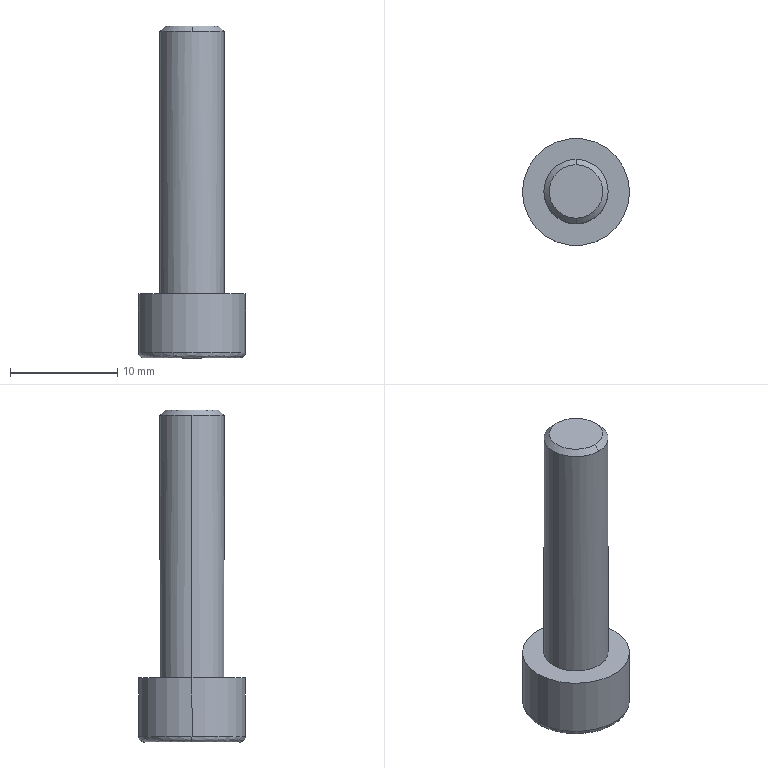Part | SolidWorks | features BaseBody 1 | 1 solid | 25 faces | box 10 x 10 x 31 mm | volume 1100 mm3 | plane 15 | cylinder 4 | cone 4 | spline 2 | commonest cylinder face diameters 6 x2 10 x2
STEP:
#1=CARTESIAN_POINT('',(-5.,0.,0.5));
#2=VERTEX_POINT('',#1);
#3=CARTESIAN_POINT('',(5.,0.,0.5));
#4=VERTEX_POINT('',#3);
#5=CARTESIAN_POINT('',(0.,0.,0.5));
#6=DIRECTION('',(0.,0.,1.));
#7=DIRECTION('',(-1.,0.,0.));
#8=AXIS2_PLACEMENT_3D('',#5,#6,#7);
#9=CIRCLE('',#8,5.);
#10=EDGE_CURVE('',#2,#4,#9,.T.);
#11=ORIENTED_EDGE('',*,*,#10,.F.);
#12=CARTESIAN_POINT('',(-4.5,0.,0.));
#13=VERTEX_POINT('',#12);
#14=CARTESIAN_POINT('',(-4.5,0.,0.5));
#15=DIRECTION('',(0.,-1.,0.));
#16=DIRECTION('',(-1.,0.,0.));
#17=AXIS2_PLACEMENT_3D('',#14,#15,#16);
#18=CIRCLE('',#17,0.5);
#19=EDGE_CURVE('',#2,#13,#18,.T.);
#20=ORIENTED_EDGE('',*,*,#19,.T.);
#21=CARTESIAN_POINT('',(4.5,0.,0.));
#22=VERTEX_POINT('',#21);
#23=CARTESIAN_POINT('',(-4.5,0.,0.));
#24=CARTESIAN_POINT('',(-4.5,-9.,0.));
#25=CARTESIAN_POINT('',(4.5,-9.,0.));
#26=CARTESIAN_POINT('',(4.5,0.,0.));
#27=(BOUNDED_CURVE()B_SPLINE_CURVE(3,(#23,#24,#25,#26),.UNSPECIFIED.,.F.,.F.)B_SPLINE_CURVE_WITH_KNOTS((4,4),(0.,1.),.UNSPECIFIED.)CURVE()GEOMETRIC_REPRESENTATION_ITEM()RATIONAL_B_SPLINE_CURVE((1.,0.3333,0.3333,1.))REPRESENTATION_ITEM(''));
#28=EDGE_CURVE('',#13,#22,#27,.T.);
#29=ORIENTED_EDGE('',*,*,#28,.T.);
#30=CARTESIAN_POINT('',(4.5,0.,0.5));
#31=DIRECTION('',(0.,1.,0.));
#32=DIRECTION('',(1.,0.,0.));
#33=AXIS2_PLACEMENT_3D('',#30,#31,#32);
#34=CIRCLE('',#33,0.5);
#35=EDGE_CURVE('',#4,#22,#34,.T.);
#36=ORIENTED_EDGE('',*,*,#35,.F.);
#37=EDGE_LOOP('',(#11,#20,#29,#36));
#38=FACE_OUTER_BOUND('',#37,.T.);
#39=CARTESIAN_POINT('',(-5.,0.,0.5));
#40=CARTESIAN_POINT('',(-5.,-10.,0.5));
#41=CARTESIAN_POINT('',(5.,-10.,0.5));
#42=CARTESIAN_POINT('',(5.,0.,0.5));
#43=CARTESIAN_POINT('',(-5.,0.,0.2071));
#44=CARTESIAN_POINT('',(-5.,-10.,0.2071));
#45=CARTESIAN_POINT('',(5.,-10.,0.2071));
#46=CARTESIAN_POINT('',(5.,0.,0.2071));
#47=CARTESIAN_POINT('',(-4.793,0.,0.));
#48=CARTESIAN_POINT('',(-4.793,-9.586,0.));
#49=CARTESIAN_POINT('',(4.793,-9.586,0.));
#50=CARTESIAN_POINT('',(4.793,0.,0.));
#51=CARTESIAN_POINT('',(-4.5,0.,0.));
#52=CARTESIAN_POINT('',(-4.5,-9.,0.));
#53=CARTESIAN_POINT('',(4.5,-9.,0.));
#54=CARTESIAN_POINT('',(4.5,0.,0.));
#55=(BOUNDED_SURFACE()B_SPLINE_SURFACE(3,3,((#39,#40,#41,#42),(#43,#44,#45,#46),(#47,#48,#49,#50),(#51,#52,#53,#54)),.UNSPECIFIED.,.F.,.F.,.T.)B_SPLINE_SURFACE_WITH_KNOTS((4,4),(4,4),(0.,1.),(0.,1.),.UNSPECIFIED.)GEOMETRIC_REPRESENTATION_ITEM()RATIONAL_B_SPLINE_SURFACE(((1.,0.3333,0.3333,1.),(0.8047,0.2682,0.2682,0.8047),(0.8047,0.2682,0.2682,0.8047),(1.,0.3333,0.3333,1.)))REPRESENTATION_ITEM('')SURFACE());
#56=ADVANCED_FACE('',(#38),#55,.T.);
#57=CARTESIAN_POINT('',(0.,3.,30.5));
#58=VERTEX_POINT('',#57);
#59=CARTESIAN_POINT('',(3.,0.,30.5));
#60=VERTEX_POINT('',#59);
#61=CARTESIAN_POINT('',(0.,0.,30.5));
#62=DIRECTION('',(0.,0.,-1.));
#63=DIRECTION('',(-1.,0.,0.));
#64=AXIS2_PLACEMENT_3D('',#61,#62,#63);
#65=CIRCLE('',#64,3.);
#66=EDGE_CURVE('',#58,#60,#65,.T.);
#67=ORIENTED_EDGE('',*,*,#66,.T.);
#68=CARTESIAN_POINT('',(3.,0.,6.));
#69=VERTEX_POINT('',#68);
#70=CARTESIAN_POINT('',(3.,0.,31.));
#71=DIRECTION('',(0.,0.,-1.));
#72=VECTOR('',#71,1000.);
#73=LINE('',#70,#72);
#74=EDGE_CURVE('',#60,#69,#73,.T.);
#75=ORIENTED_EDGE('',*,*,#74,.T.);
#76=CARTESIAN_POINT('',(-3.,0.,6.));
#77=VERTEX_POINT('',#76);
#78=CARTESIAN_POINT('',(0.,0.,6.));
#79=DIRECTION('',(0.,0.,1.));
#80=DIRECTION('',(-1.,0.,0.));
#81=AXIS2_PLACEMENT_3D('',#78,#79,#80);
#82=CIRCLE('',#81,3.);
#83=EDGE_CURVE('',#69,#77,#82,.T.);
#84=ORIENTED_EDGE('',*,*,#83,.T.);
#85=CARTESIAN_POINT('',(-3.,0.,30.5));
#86=VERTEX_POINT('',#85);
#87=CARTESIAN_POINT('',(-3.,0.,31.));
#88=DIRECTION('',(0.,0.,-1.));
#89=VECTOR('',#88,1000.);
#90=LINE('',#87,#89);
#91=EDGE_CURVE('',#86,#77,#90,.T.);
#92=ORIENTED_EDGE('',*,*,#91,.F.);
#93=CARTESIAN_POINT('',(0.,0.,30.5));
#94=DIRECTION('',(0.,0.,-1.));
#95=DIRECTION('',(-1.,0.,0.));
#96=AXIS2_PLACEMENT_3D('',#93,#94,#95);
#97=CIRCLE('',#96,3.);
#98=EDGE_CURVE('',#86,#58,#97,.T.);
#99=ORIENTED_EDGE('',*,*,#98,.T.);
#100=EDGE_LOOP('',(#67,#75,#84,#92,#99));
#101=FACE_OUTER_BOUND('',#100,.T.);
#102=CARTESIAN_POINT('',(0.,0.,31.));
#103=DIRECTION('',(0.,0.,-1.));
#104=DIRECTION('',(-1.,0.,0.));
#105=AXIS2_PLACEMENT_3D('',#102,#103,#104);
#106=CYLINDRICAL_SURFACE('',#105,3.);
#107=ADVANCED_FACE('',(#101),#106,.T.);
#108=CARTESIAN_POINT('',(0.,2.5,31.));
#109=VERTEX_POINT('',#108);
#110=CARTESIAN_POINT('',(0.,-2.5,31.));
#111=VERTEX_POINT('',#110);
#112=CARTESIAN_POINT('',(0.,0.,31.));
#113=DIRECTION('',(0.,0.,-1.));
#114=DIRECTION('',(0.,1.,0.));
#115=AXIS2_PLACEMENT_3D('',#112,#113,#114);
#116=CIRCLE('',#115,2.5);
#117=EDGE_CURVE('',#109,#111,#116,.T.);
#118=ORIENTED_EDGE('',*,*,#117,.T.);
#119=CARTESIAN_POINT('',(0.,-3.,30.5));
#120=VERTEX_POINT('',#119);
#121=CARTESIAN_POINT('',(0.,-3.,30.5));
#122=DIRECTION('',(0.,-0.7071,-0.7071));
#123=VECTOR('',#122,1000.);
#124=LINE('',#121,#123);
#125=EDGE_CURVE('',#111,#120,#124,.T.);
#126=ORIENTED_EDGE('',*,*,#125,.T.);
#127=CARTESIAN_POINT('',(0.,0.,30.5));
#128=DIRECTION('',(0.,0.,-1.));
#129=DIRECTION('',(-1.,0.,0.));
#130=AXIS2_PLACEMENT_3D('',#127,#128,#129);
#131=CIRCLE('',#130,3.);
#132=EDGE_CURVE('',#60,#120,#131,.T.);
#133=ORIENTED_EDGE('',*,*,#132,.F.);
#134=ORIENTED_EDGE('',*,*,#66,.F.);
#135=CARTESIAN_POINT('',(0.,3.,30.5));
#136=DIRECTION('',(0.,0.7071,-0.7071));
#137=VECTOR('',#136,1000.);
#138=LINE('',#135,#137);
#139=EDGE_CURVE('',#109,#58,#138,.T.);
#140=ORIENTED_EDGE('',*,*,#139,.F.);
#141=EDGE_LOOP('',(#118,#126,#133,#134,#140));
#142=FACE_OUTER_BOUND('',#141,.T.);
#143=CARTESIAN_POINT('',(0.,0.,30.5));
#144=DIRECTION('',(0.,0.,-1.));
#145=DIRECTION('',(0.,1.,0.));
#146=AXIS2_PLACEMENT_3D('',#143,#144,#145);
#147=CONICAL_SURFACE('',#146,3.,0.7854);
#148=ADVANCED_FACE('',(#142),#147,.T.);
#149=CARTESIAN_POINT('',(5.,0.,6.));
#150=VERTEX_POINT('',#149);
#151=CARTESIAN_POINT('',(-5.,0.,6.));
#152=VERTEX_POINT('',#151);
#153=CARTESIAN_POINT('',(0.,0.,6.));
#154=DIRECTION('',(0.,0.,1.));
#155=DIRECTION('',(-1.,0.,0.));
#156=AXIS2_PLACEMENT_3D('',#153,#154,#155);
#157=CIRCLE('',#156,5.);
#158=EDGE_CURVE('',#150,#152,#157,.T.);
#159=ORIENTED_EDGE('',*,*,#158,.F.);
#160=CARTESIAN_POINT('',(5.,0.,6.));
#161=DIRECTION('',(0.,0.,-1.));
#162=VECTOR('',#161,1000.);
#163=LINE('',#160,#162);
#164=EDGE_CURVE('',#150,#4,#163,.T.);
#165=ORIENTED_EDGE('',*,*,#164,.T.);
#166=CARTESIAN_POINT('',(0.,0.,0.5));
#167=DIRECTION('',(0.,0.,1.));
#168=DIRECTION('',(-1.,0.,0.));
#169=AXIS2_PLACEMENT_3D('',#166,#167,#168);
#170=CIRCLE('',#169,5.);
#171=EDGE_CURVE('',#4,#2,#170,.T.);
#172=ORIENTED_EDGE('',*,*,#171,.T.);
#173=CARTESIAN_POINT('',(-5.,0.,6.));
#174=DIRECTION('',(0.,0.,-1.));
#175=VECTOR('',#174,1000.);
#176=LINE('',#173,#175);
#177=EDGE_CURVE('',#152,#2,#176,.T.);
#178=ORIENTED_EDGE('',*,*,#177,.F.);
#179=EDGE_LOOP('',(#159,#165,#172,#178));
#180=FACE_OUTER_BOUND('',#179,.T.);
#181=CARTESIAN_POINT('',(0.,0.,6.));
#182=DIRECTION('',(0.,0.,-1.));
#183=DIRECTION('',(-1.,0.,0.));
#184=AXIS2_PLACEMENT_3D('',#181,#182,#183);
#185=CYLINDRICAL_SURFACE('',#184,5.);
#186=ADVANCED_FACE('',(#180),#185,.T.);
#187=CARTESIAN_POINT('',(0.,0.,4.443));
#188=VERTEX_POINT('',#187);
#189=CARTESIAN_POINT('',(-2.5,0.,3.));
#190=VERTEX_POINT('',#189);
#191=CARTESIAN_POINT('',(-2.5,0.,3.));
#192=DIRECTION('',(-0.866,0.,-0.5));
#193=VECTOR('',#192,1000.);
#194=LINE('',#191,#193);
#195=EDGE_CURVE('',#188,#190,#194,.T.);
#196=ORIENTED_EDGE('',*,*,#195,.F.);
#197=CARTESIAN_POINT('',(2.5,0.,3.));
#198=VERTEX_POINT('',#197);
#199=CARTESIAN_POINT('',(2.5,0.,3.));
#200=DIRECTION('',(0.866,0.,-0.5));
#201=VECTOR('',#200,1000.);
#202=LINE('',#199,#201);
#203=EDGE_CURVE('',#188,#198,#202,.T.);
#204=ORIENTED_EDGE('',*,*,#203,.T.);
#205=CARTESIAN_POINT('',(2.165,-1.25,3.));
#206=VERTEX_POINT('',#205);
#207=CARTESIAN_POINT('',(0.,0.,3.));
#208=DIRECTION('',(0.,0.,1.));
#209=DIRECTION('',(-1.,0.,0.));
#210=AXIS2_PLACEMENT_3D('',#207,#208,#209);
#211=CIRCLE('',#210,2.5);
#212=EDGE_CURVE('',#206,#198,#211,.T.);
#213=ORIENTED_EDGE('',*,*,#212,.F.);
#214=CARTESIAN_POINT('',(0.,-2.5,3.));
#215=VERTEX_POINT('',#214);
#216=CARTESIAN_POINT('',(0.,0.,3.));
#217=DIRECTION('',(0.,0.,1.));
#218=DIRECTION('',(-1.,0.,0.));
#219=AXIS2_PLACEMENT_3D('',#216,#217,#218);
#220=CIRCLE('',#219,2.5);
#221=EDGE_CURVE('',#215,#206,#220,.T.);
#222=ORIENTED_EDGE('',*,*,#221,.F.);
#223=CARTESIAN_POINT('',(-2.165,-1.25,3.));
#224=VERTEX_POINT('',#223);
#225=CARTESIAN_POINT('',(0.,0.,3.));
#226=DIRECTION('',(0.,0.,1.));
#227=DIRECTION('',(-1.,0.,0.));
#228=AXIS2_PLACEMENT_3D('',#225,#226,#227);
#229=CIRCLE('',#228,2.5);
#230=EDGE_CURVE('',#224,#215,#229,.T.);
#231=ORIENTED_EDGE('',*,*,#230,.F.);
#232=CARTESIAN_POINT('',(0.,0.,3.));
#233=DIRECTION('',(0.,0.,1.));
#234=DIRECTION('',(-1.,0.,0.));
#235=AXIS2_PLACEMENT_3D('',#232,#233,#234);
#236=CIRCLE('',#235,2.5);
#237=EDGE_CURVE('',#190,#224,#236,.T.);
#238=ORIENTED_EDGE('',*,*,#237,.F.);
#239=EDGE_LOOP('',(#196,#204,#213,#222,#231,#238));
#240=FACE_OUTER_BOUND('',#239,.T.);
#241=CARTESIAN_POINT('',(0.,0.,3.));
#242=DIRECTION('',(0.,0.,-1.));
#243=DIRECTION('',(-1.,0.,0.));
#244=AXIS2_PLACEMENT_3D('',#241,#242,#243);
#245=CONICAL_SURFACE('',#244,2.5,1.047);
#246=ADVANCED_FACE('',(#240),#245,.F.);
#247=ORIENTED_EDGE('',*,*,#74,.F.);
#248=ORIENTED_EDGE('',*,*,#132,.T.);
#249=CARTESIAN_POINT('',(0.,0.,30.5));
#250=DIRECTION('',(0.,0.,-1.));
#251=DIRECTION('',(-1.,0.,0.));
#252=AXIS2_PLACEMENT_3D('',#249,#250,#251);
#253=CIRCLE('',#252,3.);
#254=EDGE_CURVE('',#120,#86,#253,.T.);
#255=ORIENTED_EDGE('',*,*,#254,.T.);
#256=ORIENTED_EDGE('',*,*,#91,.T.);
#257=CARTESIAN_POINT('',(0.,0.,6.));
#258=DIRECTION('',(0.,0.,1.));
#259=DIRECTION('',(-1.,0.,0.));
#260=AXIS2_PLACEMENT_3D('',#257,#258,#259);
#261=CIRCLE('',#260,3.);
#262=EDGE_CURVE('',#77,#69,#261,.T.);
#263=ORIENTED_EDGE('',*,*,#262,.T.);
#264=EDGE_LOOP('',(#247,#248,#255,#256,#263));
#265=FACE_OUTER_BOUND('',#264,.T.);
#266=CARTESIAN_POINT('',(0.,0.,31.));
#267=DIRECTION('',(0.,0.,-1.));
#268=DIRECTION('',(-1.,0.,0.));
#269=AXIS2_PLACEMENT_3D('',#266,#267,#268);
#270=CYLINDRICAL_SURFACE('',#269,3.);
#271=ADVANCED_FACE('',(#265),#270,.T.);
#272=ORIENTED_EDGE('',*,*,#262,.F.);
#273=ORIENTED_EDGE('',*,*,#83,.F.);
#274=EDGE_LOOP('',(#272,#273));
#275=FACE_BOUND('',#274,.T.);
#276=CARTESIAN_POINT('',(0.,0.,6.));
#277=DIRECTION('',(0.,0.,1.));
#278=DIRECTION('',(-1.,0.,0.));
#279=AXIS2_PLACEMENT_3D('',#276,#277,#278);
#280=CIRCLE('',#279,5.);
#281=EDGE_CURVE('',#152,#150,#280,.T.);
#282=ORIENTED_EDGE('',*,*,#281,.T.);
#283=ORIENTED_EDGE('',*,*,#158,.T.);
#284=EDGE_LOOP('',(#282,#283));
#285=FACE_OUTER_BOUND('',#284,.T.);
#286=CARTESIAN_POINT('',(0.,0.,6.));
#287=DIRECTION('',(0.,0.,1.));
#288=DIRECTION('',(1.,0.,0.));
#289=AXIS2_PLACEMENT_3D('',#286,#287,#288);
#290=PLANE('',#289);
#291=ADVANCED_FACE('',(#275,#285),#290,.T.);
#292=ORIENTED_EDGE('',*,*,#125,.F.);
#293=CARTESIAN_POINT('',(0.,0.,31.));
#294=DIRECTION('',(0.,0.,-1.));
#295=DIRECTION('',(0.,1.,0.));
#296=AXIS2_PLACEMENT_3D('',#293,#294,#295);
#297=CIRCLE('',#296,2.5);
#298=EDGE_CURVE('',#111,#109,#297,.T.);
#299=ORIENTED_EDGE('',*,*,#298,.T.);
#300=ORIENTED_EDGE('',*,*,#139,.T.);
#301=ORIENTED_EDGE('',*,*,#98,.F.);
#302=ORIENTED_EDGE('',*,*,#254,.F.);
#303=EDGE_LOOP('',(#292,#299,#300,#301,#302));
#304=FACE_OUTER_BOUND('',#303,.T.);
#305=CARTESIAN_POINT('',(0.,0.,30.5));
#306=DIRECTION('',(0.,0.,-1.));
#307=DIRECTION('',(0.,1.,0.));
#308=AXIS2_PLACEMENT_3D('',#305,#306,#307);
#309=CONICAL_SURFACE('',#308,3.,0.7854);
#310=ADVANCED_FACE('',(#304),#309,.T.);
#311=ORIENTED_EDGE('',*,*,#164,.F.);
#312=ORIENTED_EDGE('',*,*,#281,.F.);
#313=ORIENTED_EDGE('',*,*,#177,.T.);
#314=ORIENTED_EDGE('',*,*,#10,.T.);
#315=EDGE_LOOP('',(#311,#312,#313,#314));
#316=FACE_OUTER_BOUND('',#315,.T.);
#317=CARTESIAN_POINT('',(0.,0.,6.));
#318=DIRECTION('',(0.,0.,-1.));
#319=DIRECTION('',(-1.,0.,0.));
#320=AXIS2_PLACEMENT_3D('',#317,#318,#319);
#321=CYLINDRICAL_SURFACE('',#320,5.);
#322=ADVANCED_FACE('',(#316),#321,.T.);
#323=ORIENTED_EDGE('',*,*,#117,.F.);
#324=ORIENTED_EDGE('',*,*,#298,.F.);
#325=EDGE_LOOP('',(#323,#324));
#326=FACE_OUTER_BOUND('',#325,.T.);
#327=CARTESIAN_POINT('',(0.,0.,31.));
#328=DIRECTION('',(0.,0.,1.));
#329=DIRECTION('',(1.,0.,0.));
#330=AXIS2_PLACEMENT_3D('',#327,#328,#329);
#331=PLANE('',#330);
#332=ADVANCED_FACE('',(#326),#331,.T.);
#333=ORIENTED_EDGE('',*,*,#19,.F.);
#334=ORIENTED_EDGE('',*,*,#171,.F.);
#335=ORIENTED_EDGE('',*,*,#35,.T.);
#336=CARTESIAN_POINT('',(4.5,0.,0.));
#337=CARTESIAN_POINT('',(4.5,9.,0.));
#338=CARTESIAN_POINT('',(-4.5,9.,0.));
#339=CARTESIAN_POINT('',(-4.5,0.,0.));
#340=(BOUNDED_CURVE()B_SPLINE_CURVE(3,(#336,#337,#338,#339),.UNSPECIFIED.,.F.,.F.)B_SPLINE_CURVE_WITH_KNOTS((4,4),(0.,1.),.UNSPECIFIED.)CURVE()GEOMETRIC_REPRESENTATION_ITEM()RATIONAL_B_SPLINE_CURVE((1.,0.3333,0.3333,1.))REPRESENTATION_ITEM(''));
#341=EDGE_CURVE('',#22,#13,#340,.T.);
#342=ORIENTED_EDGE('',*,*,#341,.T.);
#343=EDGE_LOOP('',(#333,#334,#335,#342));
#344=FACE_OUTER_BOUND('',#343,.T.);
#345=CARTESIAN_POINT('',(5.,0.,0.5));
#346=CARTESIAN_POINT('',(5.,10.,0.5));
#347=CARTESIAN_POINT('',(-5.,10.,0.5));
#348=CARTESIAN_POINT('',(-5.,0.,0.5));
#349=CARTESIAN_POINT('',(5.,0.,0.2071));
#350=CARTESIAN_POINT('',(5.,10.,0.2071));
#351=CARTESIAN_POINT('',(-5.,10.,0.2071));
#352=CARTESIAN_POINT('',(-5.,0.,0.2071));
#353=CARTESIAN_POINT('',(4.793,0.,0.));
#354=CARTESIAN_POINT('',(4.793,9.586,0.));
#355=CARTESIAN_POINT('',(-4.793,9.586,0.));
#356=CARTESIAN_POINT('',(-4.793,0.,0.));
#357=CARTESIAN_POINT('',(4.5,0.,0.));
#358=CARTESIAN_POINT('',(4.5,9.,0.));
#359=CARTESIAN_POINT('',(-4.5,9.,0.));
#360=CARTESIAN_POINT('',(-4.5,0.,0.));
#361=(BOUNDED_SURFACE()B_SPLINE_SURFACE(3,3,((#345,#346,#347,#348),(#349,#350,#351,#352),(#353,#354,#355,#356),(#357,#358,#359,#360)),.UNSPECIFIED.,.F.,.F.,.T.)B_SPLINE_SURFACE_WITH_KNOTS((4,4),(4,4),(0.,1.),(0.,1.),.UNSPECIFIED.)GEOMETRIC_REPRESENTATION_ITEM()RATIONAL_B_SPLINE_SURFACE(((1.,0.3333,0.3333,1.),(0.8047,0.2682,0.2682,0.8047),(0.8047,0.2682,0.2682,0.8047),(1.,0.3333,0.3333,1.)))REPRESENTATION_ITEM('')SURFACE());
#362=ADVANCED_FACE('',(#344),#361,.T.);
#363=ORIENTED_EDGE('',*,*,#341,.F.);
#364=ORIENTED_EDGE('',*,*,#28,.F.);
#365=EDGE_LOOP('',(#363,#364));
#366=FACE_OUTER_BOUND('',#365,.T.);
#367=CARTESIAN_POINT('',(-2.887,0.,0.));
#368=VERTEX_POINT('',#367);
#369=CARTESIAN_POINT('',(-1.443,2.5,0.));
#370=VERTEX_POINT('',#369);
#371=CARTESIAN_POINT('',(-2.887,0.,0.));
#372=DIRECTION('',(0.5,0.866,0.));
#373=VECTOR('',#372,1000.);
#374=LINE('',#371,#373);
#375=EDGE_CURVE('',#368,#370,#374,.T.);
#376=ORIENTED_EDGE('',*,*,#375,.F.);
#377=CARTESIAN_POINT('',(-1.443,-2.5,0.));
#378=VERTEX_POINT('',#377);
#379=CARTESIAN_POINT('',(-1.443,-2.5,0.));
#380=DIRECTION('',(-0.5,0.866,0.));
#381=VECTOR('',#380,1000.);
#382=LINE('',#379,#381);
#383=EDGE_CURVE('',#378,#368,#382,.T.);
#384=ORIENTED_EDGE('',*,*,#383,.F.);
#385=CARTESIAN_POINT('',(1.443,-2.5,0.));
#386=VERTEX_POINT('',#385);
#387=CARTESIAN_POINT('',(0.,-2.5,0.));
#388=DIRECTION('',(-1.,0.,0.));
#389=VECTOR('',#388,1000.);
#390=LINE('',#387,#389);
#391=EDGE_CURVE('',#386,#378,#390,.T.);
#392=ORIENTED_EDGE('',*,*,#391,.F.);
#393=CARTESIAN_POINT('',(2.887,0.,0.));
#394=VERTEX_POINT('',#393);
#395=CARTESIAN_POINT('',(2.887,0.,0.));
#396=DIRECTION('',(-0.5,-0.866,0.));
#397=VECTOR('',#396,1000.);
#398=LINE('',#395,#397);
#399=EDGE_CURVE('',#394,#386,#398,.T.);
#400=ORIENTED_EDGE('',*,*,#399,.F.);
#401=CARTESIAN_POINT('',(1.443,2.5,0.));
#402=VERTEX_POINT('',#401);
#403=CARTESIAN_POINT('',(1.443,2.5,0.));
#404=DIRECTION('',(0.5,-0.866,0.));
#405=VECTOR('',#404,1000.);
#406=LINE('',#403,#405);
#407=EDGE_CURVE('',#402,#394,#406,.T.);
#408=ORIENTED_EDGE('',*,*,#407,.F.);
#409=CARTESIAN_POINT('',(0.,2.5,0.));
#410=DIRECTION('',(1.,0.,0.));
#411=VECTOR('',#410,1000.);
#412=LINE('',#409,#411);
#413=EDGE_CURVE('',#370,#402,#412,.T.);
#414=ORIENTED_EDGE('',*,*,#413,.F.);
#415=EDGE_LOOP('',(#376,#384,#392,#400,#408,#414));
#416=FACE_BOUND('',#415,.T.);
#417=CARTESIAN_POINT('',(0.,0.,0.));
#418=DIRECTION('',(0.,0.,1.));
#419=DIRECTION('',(1.,0.,0.));
#420=AXIS2_PLACEMENT_3D('',#417,#418,#419);
#421=PLANE('',#420);
#422=ADVANCED_FACE('',(#366,#416),#421,.F.);
#423=CARTESIAN_POINT('',(1.443,2.5,3.));
#424=VERTEX_POINT('',#423);
#425=CARTESIAN_POINT('',(1.443,2.5,3.));
#426=DIRECTION('',(0.,0.,-1.));
#427=VECTOR('',#426,1000.);
#428=LINE('',#425,#427);
#429=EDGE_CURVE('',#424,#402,#428,.T.);
#430=ORIENTED_EDGE('',*,*,#429,.F.);
#431=CARTESIAN_POINT('',(0.,2.5,3.));
#432=VERTEX_POINT('',#431);
#433=CARTESIAN_POINT('',(0.,2.5,3.));
#434=DIRECTION('',(1.,0.,0.));
#435=VECTOR('',#434,1000.);
#436=LINE('',#433,#435);
#437=EDGE_CURVE('',#432,#424,#436,.T.);
#438=ORIENTED_EDGE('',*,*,#437,.F.);
#439=CARTESIAN_POINT('',(-1.443,2.5,3.));
#440=VERTEX_POINT('',#439);
#441=CARTESIAN_POINT('',(0.,2.5,3.));
#442=DIRECTION('',(1.,0.,0.));
#443=VECTOR('',#442,1000.);
#444=LINE('',#441,#443);
#445=EDGE_CURVE('',#440,#432,#444,.T.);
#446=ORIENTED_EDGE('',*,*,#445,.F.);
#447=CARTESIAN_POINT('',(-1.443,2.5,3.));
#448=DIRECTION('',(0.,0.,1.));
#449=VECTOR('',#448,1000.);
#450=LINE('',#447,#449);
#451=EDGE_CURVE('',#370,#440,#450,.T.);
#452=ORIENTED_EDGE('',*,*,#451,.F.);
#453=ORIENTED_EDGE('',*,*,#413,.T.);
#454=EDGE_LOOP('',(#430,#438,#446,#452,#453));
#455=FACE_OUTER_BOUND('',#454,.T.);
#456=CARTESIAN_POINT('',(-1.443,2.5,3.));
#457=DIRECTION('',(0.,1.,0.));
#458=DIRECTION('',(0.,0.,1.));
#459=AXIS2_PLACEMENT_3D('',#456,#457,#458);
#460=PLANE('',#459);
#461=ADVANCED_FACE('',(#455),#460,.F.);
#462=ORIENTED_EDGE('',*,*,#451,.T.);
#463=CARTESIAN_POINT('',(-2.165,1.25,3.));
#464=VERTEX_POINT('',#463);
#465=CARTESIAN_POINT('',(-2.165,1.25,3.));
#466=DIRECTION('',(0.5,0.866,0.));
#467=VECTOR('',#466,1000.);
#468=LINE('',#465,#467);
#469=EDGE_CURVE('',#464,#440,#468,.T.);
#470=ORIENTED_EDGE('',*,*,#469,.F.);
#471=CARTESIAN_POINT('',(-2.887,0.,3.));
#472=VERTEX_POINT('',#471);
#473=CARTESIAN_POINT('',(-2.887,0.,3.));
#474=DIRECTION('',(0.5,0.866,0.));
#475=VECTOR('',#474,1000.);
#476=LINE('',#473,#475);
#477=EDGE_CURVE('',#472,#464,#476,.T.);
#478=ORIENTED_EDGE('',*,*,#477,.F.);
#479=CARTESIAN_POINT('',(-2.887,0.,3.));
#480=DIRECTION('',(0.,0.,1.));
#481=VECTOR('',#480,1000.);
#482=LINE('',#479,#481);
#483=EDGE_CURVE('',#368,#472,#482,.T.);
#484=ORIENTED_EDGE('',*,*,#483,.F.);
#485=ORIENTED_EDGE('',*,*,#375,.T.);
#486=EDGE_LOOP('',(#462,#470,#478,#484,#485));
#487=FACE_OUTER_BOUND('',#486,.T.);
#488=CARTESIAN_POINT('',(-2.887,0.,3.));
#489=DIRECTION('',(-0.866,0.5,0.));
#490=DIRECTION('',(-0.5,-0.866,0.));
#491=AXIS2_PLACEMENT_3D('',#488,#489,#490);
#492=PLANE('',#491);
#493=ADVANCED_FACE('',(#487),#492,.F.);
#494=ORIENTED_EDGE('',*,*,#483,.T.);
#495=CARTESIAN_POINT('',(-1.443,-2.5,3.));
#496=DIRECTION('',(-0.5,0.866,0.));
#497=VECTOR('',#496,1000.);
#498=LINE('',#495,#497);
#499=EDGE_CURVE('',#224,#472,#498,.T.);
#500=ORIENTED_EDGE('',*,*,#499,.F.);
#501=CARTESIAN_POINT('',(-1.443,-2.5,3.));
#502=VERTEX_POINT('',#501);
#503=CARTESIAN_POINT('',(-1.443,-2.5,3.));
#504=DIRECTION('',(-0.5,0.866,0.));
#505=VECTOR('',#504,1000.);
#506=LINE('',#503,#505);
#507=EDGE_CURVE('',#502,#224,#506,.T.);
#508=ORIENTED_EDGE('',*,*,#507,.F.);
#509=CARTESIAN_POINT('',(-1.443,-2.5,3.));
#510=DIRECTION('',(0.,0.,1.));
#511=VECTOR('',#510,1000.);
#512=LINE('',#509,#511);
#513=EDGE_CURVE('',#378,#502,#512,.T.);
#514=ORIENTED_EDGE('',*,*,#513,.F.);
#515=ORIENTED_EDGE('',*,*,#383,.T.);
#516=EDGE_LOOP('',(#494,#500,#508,#514,#515));
#517=FACE_OUTER_BOUND('',#516,.T.);
#518=CARTESIAN_POINT('',(-1.443,-2.5,3.));
#519=DIRECTION('',(-0.866,-0.5,0.));
#520=DIRECTION('',(0.5,-0.866,0.));
#521=AXIS2_PLACEMENT_3D('',#518,#519,#520);
#522=PLANE('',#521);
#523=ADVANCED_FACE('',(#517),#522,.F.);
#524=ORIENTED_EDGE('',*,*,#513,.T.);
#525=CARTESIAN_POINT('',(0.,-2.5,3.));
#526=DIRECTION('',(-1.,0.,0.));
#527=VECTOR('',#526,1000.);
#528=LINE('',#525,#527);
#529=EDGE_CURVE('',#215,#502,#528,.T.);
#530=ORIENTED_EDGE('',*,*,#529,.F.);
#531=CARTESIAN_POINT('',(1.443,-2.5,3.));
#532=VERTEX_POINT('',#531);
#533=CARTESIAN_POINT('',(0.,-2.5,3.));
#534=DIRECTION('',(-1.,0.,0.));
#535=VECTOR('',#534,1000.);
#536=LINE('',#533,#535);
#537=EDGE_CURVE('',#532,#215,#536,.T.);
#538=ORIENTED_EDGE('',*,*,#537,.F.);
#539=CARTESIAN_POINT('',(1.443,-2.5,3.));
#540=DIRECTION('',(0.,0.,1.));
#541=VECTOR('',#540,1000.);
#542=LINE('',#539,#541);
#543=EDGE_CURVE('',#386,#532,#542,.T.);
#544=ORIENTED_EDGE('',*,*,#543,.F.);
#545=ORIENTED_EDGE('',*,*,#391,.T.);
#546=EDGE_LOOP('',(#524,#530,#538,#544,#545));
#547=FACE_OUTER_BOUND('',#546,.T.);
#548=CARTESIAN_POINT('',(1.443,-2.5,3.));
#549=DIRECTION('',(0.,-1.,0.));
#550=DIRECTION('',(0.,0.,-1.));
#551=AXIS2_PLACEMENT_3D('',#548,#549,#550);
#552=PLANE('',#551);
#553=ADVANCED_FACE('',(#547),#552,.F.);
#554=ORIENTED_EDGE('',*,*,#543,.T.);
#555=CARTESIAN_POINT('',(2.165,-1.25,3.));
#556=DIRECTION('',(-0.5,-0.866,0.));
#557=VECTOR('',#556,1000.);
#558=LINE('',#555,#557);
#559=EDGE_CURVE('',#206,#532,#558,.T.);
#560=ORIENTED_EDGE('',*,*,#559,.F.);
#561=CARTESIAN_POINT('',(2.887,0.,3.));
#562=VERTEX_POINT('',#561);
#563=CARTESIAN_POINT('',(2.887,0.,3.));
#564=DIRECTION('',(-0.5,-0.866,0.));
#565=VECTOR('',#564,1000.);
#566=LINE('',#563,#565);
#567=EDGE_CURVE('',#562,#206,#566,.T.);
#568=ORIENTED_EDGE('',*,*,#567,.F.);
#569=CARTESIAN_POINT('',(2.887,0.,3.));
#570=DIRECTION('',(0.,0.,1.));
#571=VECTOR('',#570,1000.);
#572=LINE('',#569,#571);
#573=EDGE_CURVE('',#394,#562,#572,.T.);
#574=ORIENTED_EDGE('',*,*,#573,.F.);
#575=ORIENTED_EDGE('',*,*,#399,.T.);
#576=EDGE_LOOP('',(#554,#560,#568,#574,#575));
#577=FACE_OUTER_BOUND('',#576,.T.);
#578=CARTESIAN_POINT('',(2.887,0.,3.));
#579=DIRECTION('',(0.866,-0.5,0.));
#580=DIRECTION('',(0.5,0.866,0.));
#581=AXIS2_PLACEMENT_3D('',#578,#579,#580);
#582=PLANE('',#581);
#583=ADVANCED_FACE('',(#577),#582,.F.);
#584=ORIENTED_EDGE('',*,*,#573,.T.);
#585=CARTESIAN_POINT('',(2.165,1.25,3.));
#586=VERTEX_POINT('',#585);
#587=CARTESIAN_POINT('',(1.443,2.5,3.));
#588=DIRECTION('',(0.5,-0.866,0.));
#589=VECTOR('',#588,1000.);
#590=LINE('',#587,#589);
#591=EDGE_CURVE('',#586,#562,#590,.T.);
#592=ORIENTED_EDGE('',*,*,#591,.F.);
#593=CARTESIAN_POINT('',(1.443,2.5,3.));
#594=DIRECTION('',(0.5,-0.866,0.));
#595=VECTOR('',#594,1000.);
#596=LINE('',#593,#595);
#597=EDGE_CURVE('',#424,#586,#596,.T.);
#598=ORIENTED_EDGE('',*,*,#597,.F.);
#599=ORIENTED_EDGE('',*,*,#429,.T.);
#600=ORIENTED_EDGE('',*,*,#407,.T.);
#601=EDGE_LOOP('',(#584,#592,#598,#599,#600));
#602=FACE_OUTER_BOUND('',#601,.T.);
#603=CARTESIAN_POINT('',(1.443,2.5,3.));
#604=DIRECTION('',(0.866,0.5,0.));
#605=DIRECTION('',(-0.5,0.866,0.));
#606=AXIS2_PLACEMENT_3D('',#603,#604,#605);
#607=PLANE('',#606);
#608=ADVANCED_FACE('',(#602),#607,.F.);
#609=ORIENTED_EDGE('',*,*,#477,.T.);
#610=CARTESIAN_POINT('',(0.,0.,3.));
#611=DIRECTION('',(0.,0.,1.));
#612=DIRECTION('',(-1.,0.,0.));
#613=AXIS2_PLACEMENT_3D('',#610,#611,#612);
#614=CIRCLE('',#613,2.5);
#615=EDGE_CURVE('',#464,#190,#614,.T.);
#616=ORIENTED_EDGE('',*,*,#615,.T.);
#617=ORIENTED_EDGE('',*,*,#237,.T.);
#618=ORIENTED_EDGE('',*,*,#499,.T.);
#619=EDGE_LOOP('',(#609,#616,#617,#618));
#620=FACE_OUTER_BOUND('',#619,.T.);
#621=CARTESIAN_POINT('',(0.,0.,3.));
#622=DIRECTION('',(0.,0.,-1.));
#623=DIRECTION('',(-1.,0.,0.));
#624=AXIS2_PLACEMENT_3D('',#621,#622,#623);
#625=PLANE('',#624);
#626=ADVANCED_FACE('',(#620),#625,.T.);
#627=ORIENTED_EDGE('',*,*,#567,.T.);
#628=ORIENTED_EDGE('',*,*,#212,.T.);
#629=CARTESIAN_POINT('',(0.,0.,3.));
#630=DIRECTION('',(0.,0.,1.));
#631=DIRECTION('',(-1.,0.,0.));
#632=AXIS2_PLACEMENT_3D('',#629,#630,#631);
#633=CIRCLE('',#632,2.5);
#634=EDGE_CURVE('',#198,#586,#633,.T.);
#635=ORIENTED_EDGE('',*,*,#634,.T.);
#636=ORIENTED_EDGE('',*,*,#591,.T.);
#637=EDGE_LOOP('',(#627,#628,#635,#636));
#638=FACE_OUTER_BOUND('',#637,.T.);
#639=CARTESIAN_POINT('',(0.,0.,3.));
#640=DIRECTION('',(0.,0.,-1.));
#641=DIRECTION('',(-1.,0.,0.));
#642=AXIS2_PLACEMENT_3D('',#639,#640,#641);
#643=PLANE('',#642);
#644=ADVANCED_FACE('',(#638),#643,.T.);
#645=ORIENTED_EDGE('',*,*,#437,.T.);
#646=ORIENTED_EDGE('',*,*,#597,.T.);
#647=CARTESIAN_POINT('',(0.,0.,3.));
#648=DIRECTION('',(0.,0.,1.));
#649=DIRECTION('',(-1.,0.,0.));
#650=AXIS2_PLACEMENT_3D('',#647,#648,#649);
#651=CIRCLE('',#650,2.5);
#652=EDGE_CURVE('',#586,#432,#651,.T.);
#653=ORIENTED_EDGE('',*,*,#652,.T.);
#654=EDGE_LOOP('',(#645,#646,#653));
#655=FACE_OUTER_BOUND('',#654,.T.);
#656=CARTESIAN_POINT('',(0.,0.,3.));
#657=DIRECTION('',(0.,0.,-1.));
#658=DIRECTION('',(-1.,0.,0.));
#659=AXIS2_PLACEMENT_3D('',#656,#657,#658);
#660=PLANE('',#659);
#661=ADVANCED_FACE('',(#655),#660,.T.);
#662=ORIENTED_EDGE('',*,*,#203,.F.);
#663=ORIENTED_EDGE('',*,*,#195,.T.);
#664=ORIENTED_EDGE('',*,*,#615,.F.);
#665=CARTESIAN_POINT('',(0.,0.,3.));
#666=DIRECTION('',(0.,0.,1.));
#667=DIRECTION('',(-1.,0.,0.));
#668=AXIS2_PLACEMENT_3D('',#665,#666,#667);
#669=CIRCLE('',#668,2.5);
#670=EDGE_CURVE('',#432,#464,#669,.T.);
#671=ORIENTED_EDGE('',*,*,#670,.F.);
#672=ORIENTED_EDGE('',*,*,#652,.F.);
#673=ORIENTED_EDGE('',*,*,#634,.F.);
#674=EDGE_LOOP('',(#662,#663,#664,#671,#672,#673));
#675=FACE_OUTER_BOUND('',#674,.T.);
#676=CARTESIAN_POINT('',(0.,0.,3.));
#677=DIRECTION('',(0.,0.,-1.));
#678=DIRECTION('',(-1.,0.,0.));
#679=AXIS2_PLACEMENT_3D('',#676,#677,#678);
#680=CONICAL_SURFACE('',#679,2.5,1.047);
#681=ADVANCED_FACE('',(#675),#680,.F.);
#682=ORIENTED_EDGE('',*,*,#469,.T.);
#683=ORIENTED_EDGE('',*,*,#445,.T.);
#684=ORIENTED_EDGE('',*,*,#670,.T.);
#685=EDGE_LOOP('',(#682,#683,#684));
#686=FACE_OUTER_BOUND('',#685,.T.);
#687=CARTESIAN_POINT('',(0.,0.,3.));
#688=DIRECTION('',(0.,0.,-1.));
#689=DIRECTION('',(-1.,0.,0.));
#690=AXIS2_PLACEMENT_3D('',#687,#688,#689);
#691=PLANE('',#690);
#692=ADVANCED_FACE('',(#686),#691,.T.);
#693=ORIENTED_EDGE('',*,*,#559,.T.);
#694=ORIENTED_EDGE('',*,*,#537,.T.);
#695=ORIENTED_EDGE('',*,*,#221,.T.);
#696=EDGE_LOOP('',(#693,#694,#695));
#697=FACE_OUTER_BOUND('',#696,.T.);
#698=CARTESIAN_POINT('',(0.,0.,3.));
#699=DIRECTION('',(0.,0.,-1.));
#700=DIRECTION('',(-1.,0.,0.));
#701=AXIS2_PLACEMENT_3D('',#698,#699,#700);
#702=PLANE('',#701);
#703=ADVANCED_FACE('',(#697),#702,.T.);
#704=ORIENTED_EDGE('',*,*,#529,.T.);
#705=ORIENTED_EDGE('',*,*,#507,.T.);
#706=ORIENTED_EDGE('',*,*,#230,.T.);
#707=EDGE_LOOP('',(#704,#705,#706));
#708=FACE_OUTER_BOUND('',#707,.T.);
#709=CARTESIAN_POINT('',(0.,0.,3.));
#710=DIRECTION('',(0.,0.,-1.));
#711=DIRECTION('',(-1.,0.,0.));
#712=AXIS2_PLACEMENT_3D('',#709,#710,#711);
#713=PLANE('',#712);
#714=ADVANCED_FACE('',(#708),#713,.T.);
#715=CLOSED_SHELL('',(#56,#107,#148,#186,#246,#271,#291,#310,#322,#332,#362,#422,#461,#493,#523,#553,#583,#608,#626,#644,#661,#681,#692,#703,#714));
#716=MANIFOLD_SOLID_BREP('',#715);
#717=CARTESIAN_POINT('',(0.,0.,0.));
#718=DIRECTION('',(0.,0.,1.));
#719=DIRECTION('',(1.,0.,0.));
#720=AXIS2_PLACEMENT_3D('',#717,#718,#719);
#721=(LENGTH_UNIT()NAMED_UNIT(*)SI_UNIT(.MILLI.,.METRE.));
#722=UNCERTAINTY_MEASURE_WITH_UNIT(LENGTH_MEASURE(0.00001),#721,'','');
#723=(NAMED_UNIT(*)PLANE_ANGLE_UNIT()SI_UNIT($,.RADIAN.));
#724=(NAMED_UNIT(*)SI_UNIT($,.STERADIAN.)SOLID_ANGLE_UNIT());
#725=(GEOMETRIC_REPRESENTATION_CONTEXT(3)GLOBAL_UNCERTAINTY_ASSIGNED_CONTEXT((#722))GLOBAL_UNIT_ASSIGNED_CONTEXT((#721,#723,#724))REPRESENTATION_CONTEXT('',''));
#726=ADVANCED_BREP_SHAPE_REPRESENTATION('',(#716,#720),#725);